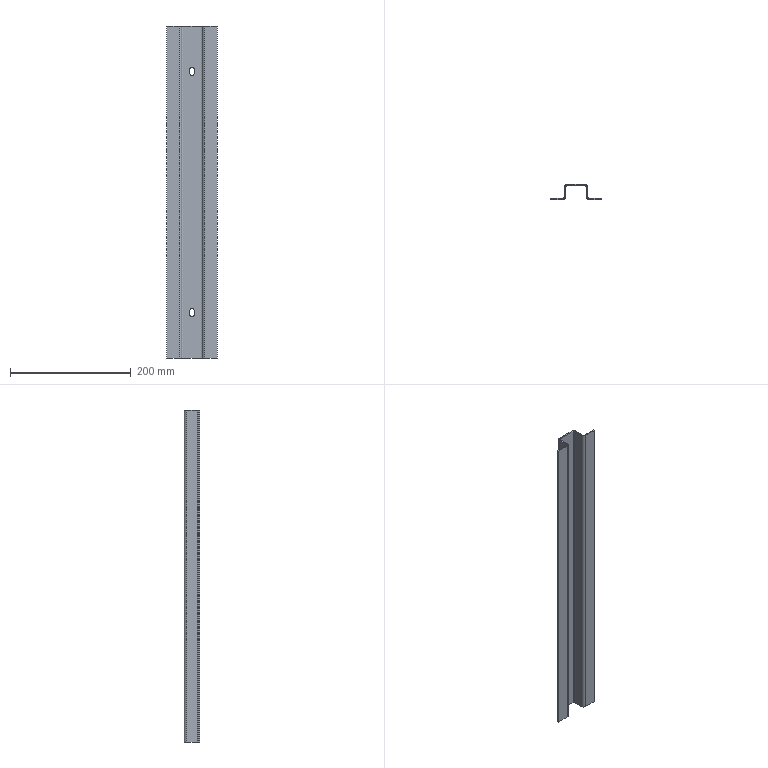Part | STEP file | SYL_0392D6J1SYL0380DJ1006_2_1-2 | 1 solid | 50 faces | box 84 x 25 x 550 mm | volume 136985 mm3 | plane 34 | cylinder 16 | commonest cylinder face diameters 7 x8 4 x4 8 x4
STEP:
#1=CARTESIAN_POINT('',(-3.5,25.,-203.5));
#2=VERTEX_POINT('',#1);
#3=CARTESIAN_POINT('',(-3.5,23.,-203.5));
#4=VERTEX_POINT('',#3);
#5=CARTESIAN_POINT('',(-3.5,23.,-203.5));
#6=DIRECTION('',(0.,-1.,0.));
#7=VECTOR('',#6,1000.);
#8=LINE('',#5,#7);
#9=EDGE_CURVE('',#2,#4,#8,.T.);
#10=ORIENTED_EDGE('',*,*,#9,.F.);
#11=CARTESIAN_POINT('',(-3.5,25.,-196.5));
#12=VERTEX_POINT('',#11);
#13=CARTESIAN_POINT('',(-3.5,25.,-275.));
#14=DIRECTION('',(0.,0.,-1.));
#15=VECTOR('',#14,1000.);
#16=LINE('',#13,#15);
#17=EDGE_CURVE('',#12,#2,#16,.T.);
#18=ORIENTED_EDGE('',*,*,#17,.F.);
#19=CARTESIAN_POINT('',(-3.5,23.,-196.5));
#20=VERTEX_POINT('',#19);
#21=CARTESIAN_POINT('',(-3.5,23.,-196.5));
#22=DIRECTION('',(0.,-1.,0.));
#23=VECTOR('',#22,1000.);
#24=LINE('',#21,#23);
#25=EDGE_CURVE('',#12,#20,#24,.T.);
#26=ORIENTED_EDGE('',*,*,#25,.T.);
#27=CARTESIAN_POINT('',(-3.5,23.,-196.5));
#28=DIRECTION('',(0.,0.,-1.));
#29=VECTOR('',#28,1000.);
#30=LINE('',#27,#29);
#31=EDGE_CURVE('',#20,#4,#30,.T.);
#32=ORIENTED_EDGE('',*,*,#31,.T.);
#33=EDGE_LOOP('',(#10,#18,#26,#32));
#34=FACE_OUTER_BOUND('',#33,.T.);
#35=CARTESIAN_POINT('',(-3.5,23.,-196.5));
#36=DIRECTION('',(-1.,0.,0.));
#37=DIRECTION('',(0.,0.,-1.));
#38=AXIS2_PLACEMENT_3D('',#35,#36,#37);
#39=PLANE('',#38);
#40=ADVANCED_FACE('',(#34),#39,.F.);
#41=ORIENTED_EDGE('',*,*,#25,.F.);
#42=CARTESIAN_POINT('',(0.,25.,-193.));
#43=VERTEX_POINT('',#42);
#44=CARTESIAN_POINT('',(0.,25.,-196.5));
#45=DIRECTION('',(0.,1.,0.));
#46=DIRECTION('',(0.,0.,1.));
#47=AXIS2_PLACEMENT_3D('',#44,#45,#46);
#48=CIRCLE('',#47,3.5);
#49=EDGE_CURVE('',#12,#43,#48,.T.);
#50=ORIENTED_EDGE('',*,*,#49,.T.);
#51=CARTESIAN_POINT('',(0.,23.,-193.));
#52=VERTEX_POINT('',#51);
#53=CARTESIAN_POINT('',(0.,23.,-193.));
#54=DIRECTION('',(0.,-1.,0.));
#55=VECTOR('',#54,1000.);
#56=LINE('',#53,#55);
#57=EDGE_CURVE('',#43,#52,#56,.T.);
#58=ORIENTED_EDGE('',*,*,#57,.T.);
#59=CARTESIAN_POINT('',(0.,23.,-196.5));
#60=DIRECTION('',(0.,1.,0.));
#61=DIRECTION('',(-1.,0.,0.));
#62=AXIS2_PLACEMENT_3D('',#59,#60,#61);
#63=CIRCLE('',#62,3.5);
#64=EDGE_CURVE('',#20,#52,#63,.T.);
#65=ORIENTED_EDGE('',*,*,#64,.F.);
#66=EDGE_LOOP('',(#41,#50,#58,#65));
#67=FACE_OUTER_BOUND('',#66,.T.);
#68=CARTESIAN_POINT('',(0.,23.,-196.5));
#69=DIRECTION('',(0.,-1.,0.));
#70=DIRECTION('',(0.,0.,-1.));
#71=AXIS2_PLACEMENT_3D('',#68,#69,#70);
#72=CYLINDRICAL_SURFACE('',#71,3.5);
#73=ADVANCED_FACE('',(#67),#72,.F.);
#74=ORIENTED_EDGE('',*,*,#57,.F.);
#75=CARTESIAN_POINT('',(3.5,25.,-196.5));
#76=VERTEX_POINT('',#75);
#77=CARTESIAN_POINT('',(0.,25.,-196.5));
#78=DIRECTION('',(0.,1.,0.));
#79=DIRECTION('',(0.,0.,1.));
#80=AXIS2_PLACEMENT_3D('',#77,#78,#79);
#81=CIRCLE('',#80,3.5);
#82=EDGE_CURVE('',#43,#76,#81,.T.);
#83=ORIENTED_EDGE('',*,*,#82,.T.);
#84=CARTESIAN_POINT('',(3.5,23.,-196.5));
#85=VERTEX_POINT('',#84);
#86=CARTESIAN_POINT('',(3.5,23.,-196.5));
#87=DIRECTION('',(0.,-1.,0.));
#88=VECTOR('',#87,1000.);
#89=LINE('',#86,#88);
#90=EDGE_CURVE('',#76,#85,#89,.T.);
#91=ORIENTED_EDGE('',*,*,#90,.T.);
#92=CARTESIAN_POINT('',(0.,23.,-196.5));
#93=DIRECTION('',(0.,1.,0.));
#94=DIRECTION('',(0.,0.,1.));
#95=AXIS2_PLACEMENT_3D('',#92,#93,#94);
#96=CIRCLE('',#95,3.5);
#97=EDGE_CURVE('',#52,#85,#96,.T.);
#98=ORIENTED_EDGE('',*,*,#97,.F.);
#99=EDGE_LOOP('',(#74,#83,#91,#98));
#100=FACE_OUTER_BOUND('',#99,.T.);
#101=CARTESIAN_POINT('',(0.,23.,-196.5));
#102=DIRECTION('',(0.,-1.,0.));
#103=DIRECTION('',(0.,0.,-1.));
#104=AXIS2_PLACEMENT_3D('',#101,#102,#103);
#105=CYLINDRICAL_SURFACE('',#104,3.5);
#106=ADVANCED_FACE('',(#100),#105,.F.);
#107=ORIENTED_EDGE('',*,*,#90,.F.);
#108=CARTESIAN_POINT('',(3.5,25.,-203.5));
#109=VERTEX_POINT('',#108);
#110=CARTESIAN_POINT('',(3.5,25.,-275.));
#111=DIRECTION('',(0.,0.,1.));
#112=VECTOR('',#111,1000.);
#113=LINE('',#110,#112);
#114=EDGE_CURVE('',#109,#76,#113,.T.);
#115=ORIENTED_EDGE('',*,*,#114,.F.);
#116=CARTESIAN_POINT('',(3.5,23.,-203.5));
#117=VERTEX_POINT('',#116);
#118=CARTESIAN_POINT('',(3.5,23.,-203.5));
#119=DIRECTION('',(0.,-1.,0.));
#120=VECTOR('',#119,1000.);
#121=LINE('',#118,#120);
#122=EDGE_CURVE('',#109,#117,#121,.T.);
#123=ORIENTED_EDGE('',*,*,#122,.T.);
#124=CARTESIAN_POINT('',(3.5,23.,-203.5));
#125=DIRECTION('',(0.,0.,1.));
#126=VECTOR('',#125,1000.);
#127=LINE('',#124,#126);
#128=EDGE_CURVE('',#117,#85,#127,.T.);
#129=ORIENTED_EDGE('',*,*,#128,.T.);
#130=EDGE_LOOP('',(#107,#115,#123,#129));
#131=FACE_OUTER_BOUND('',#130,.T.);
#132=CARTESIAN_POINT('',(3.5,23.,-203.5));
#133=DIRECTION('',(1.,0.,0.));
#134=DIRECTION('',(0.,0.,1.));
#135=AXIS2_PLACEMENT_3D('',#132,#133,#134);
#136=PLANE('',#135);
#137=ADVANCED_FACE('',(#131),#136,.F.);
#138=ORIENTED_EDGE('',*,*,#122,.F.);
#139=CARTESIAN_POINT('',(0.,25.,-207.));
#140=VERTEX_POINT('',#139);
#141=CARTESIAN_POINT('',(0.,25.,-203.5));
#142=DIRECTION('',(0.,1.,0.));
#143=DIRECTION('',(0.,0.,1.));
#144=AXIS2_PLACEMENT_3D('',#141,#142,#143);
#145=CIRCLE('',#144,3.5);
#146=EDGE_CURVE('',#109,#140,#145,.T.);
#147=ORIENTED_EDGE('',*,*,#146,.T.);
#148=CARTESIAN_POINT('',(0.,23.,-207.));
#149=VERTEX_POINT('',#148);
#150=CARTESIAN_POINT('',(0.,23.,-207.));
#151=DIRECTION('',(0.,-1.,0.));
#152=VECTOR('',#151,1000.);
#153=LINE('',#150,#152);
#154=EDGE_CURVE('',#140,#149,#153,.T.);
#155=ORIENTED_EDGE('',*,*,#154,.T.);
#156=CARTESIAN_POINT('',(0.,23.,-203.5));
#157=DIRECTION('',(0.,1.,0.));
#158=DIRECTION('',(1.,0.,0.));
#159=AXIS2_PLACEMENT_3D('',#156,#157,#158);
#160=CIRCLE('',#159,3.5);
#161=EDGE_CURVE('',#117,#149,#160,.T.);
#162=ORIENTED_EDGE('',*,*,#161,.F.);
#163=EDGE_LOOP('',(#138,#147,#155,#162));
#164=FACE_OUTER_BOUND('',#163,.T.);
#165=CARTESIAN_POINT('',(0.,23.,-203.5));
#166=DIRECTION('',(0.,-1.,0.));
#167=DIRECTION('',(0.,0.,-1.));
#168=AXIS2_PLACEMENT_3D('',#165,#166,#167);
#169=CYLINDRICAL_SURFACE('',#168,3.5);
#170=ADVANCED_FACE('',(#164),#169,.F.);
#171=CARTESIAN_POINT('',(-3.5,25.,196.5));
#172=VERTEX_POINT('',#171);
#173=CARTESIAN_POINT('',(-3.5,23.,196.5));
#174=VERTEX_POINT('',#173);
#175=CARTESIAN_POINT('',(-3.5,23.,196.5));
#176=DIRECTION('',(0.,-1.,0.));
#177=VECTOR('',#176,1000.);
#178=LINE('',#175,#177);
#179=EDGE_CURVE('',#172,#174,#178,.T.);
#180=ORIENTED_EDGE('',*,*,#179,.F.);
#181=CARTESIAN_POINT('',(-3.5,25.,203.5));
#182=VERTEX_POINT('',#181);
#183=CARTESIAN_POINT('',(-3.5,25.,-275.));
#184=DIRECTION('',(0.,0.,-1.));
#185=VECTOR('',#184,1000.);
#186=LINE('',#183,#185);
#187=EDGE_CURVE('',#182,#172,#186,.T.);
#188=ORIENTED_EDGE('',*,*,#187,.F.);
#189=CARTESIAN_POINT('',(-3.5,23.,203.5));
#190=VERTEX_POINT('',#189);
#191=CARTESIAN_POINT('',(-3.5,23.,203.5));
#192=DIRECTION('',(0.,-1.,0.));
#193=VECTOR('',#192,1000.);
#194=LINE('',#191,#193);
#195=EDGE_CURVE('',#182,#190,#194,.T.);
#196=ORIENTED_EDGE('',*,*,#195,.T.);
#197=CARTESIAN_POINT('',(-3.5,23.,203.5));
#198=DIRECTION('',(0.,0.,-1.));
#199=VECTOR('',#198,1000.);
#200=LINE('',#197,#199);
#201=EDGE_CURVE('',#190,#174,#200,.T.);
#202=ORIENTED_EDGE('',*,*,#201,.T.);
#203=EDGE_LOOP('',(#180,#188,#196,#202));
#204=FACE_OUTER_BOUND('',#203,.T.);
#205=CARTESIAN_POINT('',(-3.5,23.,203.5));
#206=DIRECTION('',(-1.,0.,0.));
#207=DIRECTION('',(0.,0.,-1.));
#208=AXIS2_PLACEMENT_3D('',#205,#206,#207);
#209=PLANE('',#208);
#210=ADVANCED_FACE('',(#204),#209,.F.);
#211=ORIENTED_EDGE('',*,*,#195,.F.);
#212=CARTESIAN_POINT('',(0.,25.,207.));
#213=VERTEX_POINT('',#212);
#214=CARTESIAN_POINT('',(0.,25.,203.5));
#215=DIRECTION('',(0.,1.,0.));
#216=DIRECTION('',(0.,0.,1.));
#217=AXIS2_PLACEMENT_3D('',#214,#215,#216);
#218=CIRCLE('',#217,3.5);
#219=EDGE_CURVE('',#182,#213,#218,.T.);
#220=ORIENTED_EDGE('',*,*,#219,.T.);
#221=CARTESIAN_POINT('',(0.,23.,207.));
#222=VERTEX_POINT('',#221);
#223=CARTESIAN_POINT('',(0.,23.,207.));
#224=DIRECTION('',(0.,-1.,0.));
#225=VECTOR('',#224,1000.);
#226=LINE('',#223,#225);
#227=EDGE_CURVE('',#213,#222,#226,.T.);
#228=ORIENTED_EDGE('',*,*,#227,.T.);
#229=CARTESIAN_POINT('',(0.,23.,203.5));
#230=DIRECTION('',(0.,1.,0.));
#231=DIRECTION('',(-1.,0.,0.));
#232=AXIS2_PLACEMENT_3D('',#229,#230,#231);
#233=CIRCLE('',#232,3.5);
#234=EDGE_CURVE('',#190,#222,#233,.T.);
#235=ORIENTED_EDGE('',*,*,#234,.F.);
#236=EDGE_LOOP('',(#211,#220,#228,#235));
#237=FACE_OUTER_BOUND('',#236,.T.);
#238=CARTESIAN_POINT('',(0.,23.,203.5));
#239=DIRECTION('',(0.,-1.,0.));
#240=DIRECTION('',(0.,0.,-1.));
#241=AXIS2_PLACEMENT_3D('',#238,#239,#240);
#242=CYLINDRICAL_SURFACE('',#241,3.5);
#243=ADVANCED_FACE('',(#237),#242,.F.);
#244=ORIENTED_EDGE('',*,*,#227,.F.);
#245=CARTESIAN_POINT('',(3.5,25.,203.5));
#246=VERTEX_POINT('',#245);
#247=CARTESIAN_POINT('',(0.,25.,203.5));
#248=DIRECTION('',(0.,1.,0.));
#249=DIRECTION('',(0.,0.,1.));
#250=AXIS2_PLACEMENT_3D('',#247,#248,#249);
#251=CIRCLE('',#250,3.5);
#252=EDGE_CURVE('',#213,#246,#251,.T.);
#253=ORIENTED_EDGE('',*,*,#252,.T.);
#254=CARTESIAN_POINT('',(3.5,23.,203.5));
#255=VERTEX_POINT('',#254);
#256=CARTESIAN_POINT('',(3.5,23.,203.5));
#257=DIRECTION('',(0.,-1.,0.));
#258=VECTOR('',#257,1000.);
#259=LINE('',#256,#258);
#260=EDGE_CURVE('',#246,#255,#259,.T.);
#261=ORIENTED_EDGE('',*,*,#260,.T.);
#262=CARTESIAN_POINT('',(0.,23.,203.5));
#263=DIRECTION('',(0.,1.,0.));
#264=DIRECTION('',(0.,0.,1.));
#265=AXIS2_PLACEMENT_3D('',#262,#263,#264);
#266=CIRCLE('',#265,3.5);
#267=EDGE_CURVE('',#222,#255,#266,.T.);
#268=ORIENTED_EDGE('',*,*,#267,.F.);
#269=EDGE_LOOP('',(#244,#253,#261,#268));
#270=FACE_OUTER_BOUND('',#269,.T.);
#271=CARTESIAN_POINT('',(0.,23.,203.5));
#272=DIRECTION('',(0.,-1.,0.));
#273=DIRECTION('',(0.,0.,-1.));
#274=AXIS2_PLACEMENT_3D('',#271,#272,#273);
#275=CYLINDRICAL_SURFACE('',#274,3.5);
#276=ADVANCED_FACE('',(#270),#275,.F.);
#277=ORIENTED_EDGE('',*,*,#260,.F.);
#278=CARTESIAN_POINT('',(3.5,25.,196.5));
#279=VERTEX_POINT('',#278);
#280=CARTESIAN_POINT('',(3.5,25.,-275.));
#281=DIRECTION('',(0.,0.,1.));
#282=VECTOR('',#281,1000.);
#283=LINE('',#280,#282);
#284=EDGE_CURVE('',#279,#246,#283,.T.);
#285=ORIENTED_EDGE('',*,*,#284,.F.);
#286=CARTESIAN_POINT('',(3.5,23.,196.5));
#287=VERTEX_POINT('',#286);
#288=CARTESIAN_POINT('',(3.5,23.,196.5));
#289=DIRECTION('',(0.,-1.,0.));
#290=VECTOR('',#289,1000.);
#291=LINE('',#288,#290);
#292=EDGE_CURVE('',#279,#287,#291,.T.);
#293=ORIENTED_EDGE('',*,*,#292,.T.);
#294=CARTESIAN_POINT('',(3.5,23.,196.5));
#295=DIRECTION('',(0.,0.,1.));
#296=VECTOR('',#295,1000.);
#297=LINE('',#294,#296);
#298=EDGE_CURVE('',#287,#255,#297,.T.);
#299=ORIENTED_EDGE('',*,*,#298,.T.);
#300=EDGE_LOOP('',(#277,#285,#293,#299));
#301=FACE_OUTER_BOUND('',#300,.T.);
#302=CARTESIAN_POINT('',(3.5,23.,196.5));
#303=DIRECTION('',(1.,0.,0.));
#304=DIRECTION('',(0.,0.,1.));
#305=AXIS2_PLACEMENT_3D('',#302,#303,#304);
#306=PLANE('',#305);
#307=ADVANCED_FACE('',(#301),#306,.F.);
#308=ORIENTED_EDGE('',*,*,#292,.F.);
#309=CARTESIAN_POINT('',(0.,25.,193.));
#310=VERTEX_POINT('',#309);
#311=CARTESIAN_POINT('',(0.,25.,196.5));
#312=DIRECTION('',(0.,1.,0.));
#313=DIRECTION('',(0.,0.,1.));
#314=AXIS2_PLACEMENT_3D('',#311,#312,#313);
#315=CIRCLE('',#314,3.5);
#316=EDGE_CURVE('',#279,#310,#315,.T.);
#317=ORIENTED_EDGE('',*,*,#316,.T.);
#318=CARTESIAN_POINT('',(0.,23.,193.));
#319=VERTEX_POINT('',#318);
#320=CARTESIAN_POINT('',(0.,23.,193.));
#321=DIRECTION('',(0.,-1.,0.));
#322=VECTOR('',#321,1000.);
#323=LINE('',#320,#322);
#324=EDGE_CURVE('',#310,#319,#323,.T.);
#325=ORIENTED_EDGE('',*,*,#324,.T.);
#326=CARTESIAN_POINT('',(0.,23.,196.5));
#327=DIRECTION('',(0.,1.,0.));
#328=DIRECTION('',(1.,0.,0.));
#329=AXIS2_PLACEMENT_3D('',#326,#327,#328);
#330=CIRCLE('',#329,3.5);
#331=EDGE_CURVE('',#287,#319,#330,.T.);
#332=ORIENTED_EDGE('',*,*,#331,.F.);
#333=EDGE_LOOP('',(#308,#317,#325,#332));
#334=FACE_OUTER_BOUND('',#333,.T.);
#335=CARTESIAN_POINT('',(0.,23.,196.5));
#336=DIRECTION('',(0.,-1.,0.));
#337=DIRECTION('',(0.,0.,-1.));
#338=AXIS2_PLACEMENT_3D('',#335,#336,#337);
#339=CYLINDRICAL_SURFACE('',#338,3.5);
#340=ADVANCED_FACE('',(#334),#339,.F.);
#341=CARTESIAN_POINT('',(-19.,21.,-275.));
#342=VERTEX_POINT('',#341);
#343=CARTESIAN_POINT('',(-17.,21.,-275.));
#344=VERTEX_POINT('',#343);
#345=CARTESIAN_POINT('',(-17.,21.,-275.));
#346=DIRECTION('',(1.,0.,0.));
#347=VECTOR('',#346,1000.);
#348=LINE('',#345,#347);
#349=EDGE_CURVE('',#342,#344,#348,.T.);
#350=ORIENTED_EDGE('',*,*,#349,.F.);
#351=CARTESIAN_POINT('',(-15.,25.,-275.));
#352=VERTEX_POINT('',#351);
#353=CARTESIAN_POINT('',(-15.,21.,-275.));
#354=DIRECTION('',(0.,0.,1.));
#355=DIRECTION('',(1.,0.,0.));
#356=AXIS2_PLACEMENT_3D('',#353,#354,#355);
#357=CIRCLE('',#356,4.);
#358=EDGE_CURVE('',#352,#342,#357,.T.);
#359=ORIENTED_EDGE('',*,*,#358,.F.);
#360=CARTESIAN_POINT('',(-15.,23.,-275.));
#361=VERTEX_POINT('',#360);
#362=CARTESIAN_POINT('',(-15.,23.,-275.));
#363=DIRECTION('',(0.,-1.,0.));
#364=VECTOR('',#363,1000.);
#365=LINE('',#362,#364);
#366=EDGE_CURVE('',#352,#361,#365,.T.);
#367=ORIENTED_EDGE('',*,*,#366,.T.);
#368=CARTESIAN_POINT('',(-15.,21.,-275.));
#369=DIRECTION('',(0.,0.,1.));
#370=DIRECTION('',(0.,1.,0.));
#371=AXIS2_PLACEMENT_3D('',#368,#369,#370);
#372=CIRCLE('',#371,2.);
#373=EDGE_CURVE('',#361,#344,#372,.T.);
#374=ORIENTED_EDGE('',*,*,#373,.T.);
#375=EDGE_LOOP('',(#350,#359,#367,#374));
#376=FACE_OUTER_BOUND('',#375,.T.);
#377=CARTESIAN_POINT('',(-15.,21.,-275.));
#378=DIRECTION('',(0.,0.,-1.));
#379=DIRECTION('',(-1.,0.,0.));
#380=AXIS2_PLACEMENT_3D('',#377,#378,#379);
#381=PLANE('',#380);
#382=ADVANCED_FACE('',(#376),#381,.T.);
#383=ORIENTED_EDGE('',*,*,#366,.F.);
#384=CARTESIAN_POINT('',(15.,25.,-275.));
#385=VERTEX_POINT('',#384);
#386=CARTESIAN_POINT('',(-15.,25.,-275.));
#387=DIRECTION('',(-1.,0.,0.));
#388=VECTOR('',#387,1000.);
#389=LINE('',#386,#388);
#390=EDGE_CURVE('',#385,#352,#389,.T.);
#391=ORIENTED_EDGE('',*,*,#390,.F.);
#392=CARTESIAN_POINT('',(15.,23.,-275.));
#393=VERTEX_POINT('',#392);
#394=CARTESIAN_POINT('',(15.,23.,-275.));
#395=DIRECTION('',(0.,-1.,0.));
#396=VECTOR('',#395,1000.);
#397=LINE('',#394,#396);
#398=EDGE_CURVE('',#385,#393,#397,.T.);
#399=ORIENTED_EDGE('',*,*,#398,.T.);
#400=CARTESIAN_POINT('',(15.,23.,-275.));
#401=DIRECTION('',(-1.,0.,0.));
#402=VECTOR('',#401,1000.);
#403=LINE('',#400,#402);
#404=EDGE_CURVE('',#393,#361,#403,.T.);
#405=ORIENTED_EDGE('',*,*,#404,.T.);
#406=EDGE_LOOP('',(#383,#391,#399,#405));
#407=FACE_OUTER_BOUND('',#406,.T.);
#408=CARTESIAN_POINT('',(15.,23.,-275.));
#409=DIRECTION('',(0.,0.,1.));
#410=DIRECTION('',(-1.,0.,0.));
#411=AXIS2_PLACEMENT_3D('',#408,#409,#410);
#412=PLANE('',#411);
#413=ADVANCED_FACE('',(#407),#412,.F.);
#414=ORIENTED_EDGE('',*,*,#398,.F.);
#415=CARTESIAN_POINT('',(19.,21.,-275.));
#416=VERTEX_POINT('',#415);
#417=CARTESIAN_POINT('',(15.,21.,-275.));
#418=DIRECTION('',(0.,0.,1.));
#419=DIRECTION('',(1.,0.,0.));
#420=AXIS2_PLACEMENT_3D('',#417,#418,#419);
#421=CIRCLE('',#420,4.);
#422=EDGE_CURVE('',#416,#385,#421,.T.);
#423=ORIENTED_EDGE('',*,*,#422,.F.);
#424=CARTESIAN_POINT('',(17.,21.,-275.));
#425=VERTEX_POINT('',#424);
#426=CARTESIAN_POINT('',(17.,21.,-275.));
#427=DIRECTION('',(-1.,0.,0.));
#428=VECTOR('',#427,1000.);
#429=LINE('',#426,#428);
#430=EDGE_CURVE('',#416,#425,#429,.T.);
#431=ORIENTED_EDGE('',*,*,#430,.T.);
#432=CARTESIAN_POINT('',(15.,21.,-275.));
#433=DIRECTION('',(0.,0.,1.));
#434=DIRECTION('',(1.,0.,0.));
#435=AXIS2_PLACEMENT_3D('',#432,#433,#434);
#436=CIRCLE('',#435,2.);
#437=EDGE_CURVE('',#425,#393,#436,.T.);
#438=ORIENTED_EDGE('',*,*,#437,.T.);
#439=EDGE_LOOP('',(#414,#423,#431,#438));
#440=FACE_OUTER_BOUND('',#439,.T.);
#441=CARTESIAN_POINT('',(15.,21.,-275.));
#442=DIRECTION('',(0.,0.,-1.));
#443=DIRECTION('',(-1.,0.,0.));
#444=AXIS2_PLACEMENT_3D('',#441,#442,#443);
#445=PLANE('',#444);
#446=ADVANCED_FACE('',(#440),#445,.T.);
#447=ORIENTED_EDGE('',*,*,#430,.F.);
#448=CARTESIAN_POINT('',(19.,4.,-275.));
#449=VERTEX_POINT('',#448);
#450=CARTESIAN_POINT('',(19.,21.,-275.));
#451=DIRECTION('',(0.,1.,0.));
#452=VECTOR('',#451,1000.);
#453=LINE('',#450,#452);
#454=EDGE_CURVE('',#449,#416,#453,.T.);
#455=ORIENTED_EDGE('',*,*,#454,.F.);
#456=CARTESIAN_POINT('',(17.,4.,-275.));
#457=VERTEX_POINT('',#456);
#458=CARTESIAN_POINT('',(17.,4.,-275.));
#459=DIRECTION('',(-1.,0.,0.));
#460=VECTOR('',#459,1000.);
#461=LINE('',#458,#460);
#462=EDGE_CURVE('',#449,#457,#461,.T.);
#463=ORIENTED_EDGE('',*,*,#462,.T.);
#464=CARTESIAN_POINT('',(17.,4.,-275.));
#465=DIRECTION('',(0.,1.,0.));
#466=VECTOR('',#465,1000.);
#467=LINE('',#464,#466);
#468=EDGE_CURVE('',#457,#425,#467,.T.);
#469=ORIENTED_EDGE('',*,*,#468,.T.);
#470=EDGE_LOOP('',(#447,#455,#463,#469));
#471=FACE_OUTER_BOUND('',#470,.T.);
#472=CARTESIAN_POINT('',(17.,4.,-275.));
#473=DIRECTION('',(0.,0.,1.));
#474=DIRECTION('',(0.,1.,0.));
#475=AXIS2_PLACEMENT_3D('',#472,#473,#474);
#476=PLANE('',#475);
#477=ADVANCED_FACE('',(#471),#476,.F.);
#478=ORIENTED_EDGE('',*,*,#462,.F.);
#479=CARTESIAN_POINT('',(21.,2.,-275.));
#480=VERTEX_POINT('',#479);
#481=CARTESIAN_POINT('',(21.,4.,-275.));
#482=DIRECTION('',(0.,0.,-1.));
#483=DIRECTION('',(1.,0.,0.));
#484=AXIS2_PLACEMENT_3D('',#481,#482,#483);
#485=CIRCLE('',#484,2.);
#486=EDGE_CURVE('',#480,#449,#485,.T.);
#487=ORIENTED_EDGE('',*,*,#486,.F.);
#488=CARTESIAN_POINT('',(21.,0.,-275.));
#489=VERTEX_POINT('',#488);
#490=CARTESIAN_POINT('',(21.,0.,-275.));
#491=DIRECTION('',(0.,-1.,0.));
#492=VECTOR('',#491,1000.);
#493=LINE('',#490,#492);
#494=EDGE_CURVE('',#480,#489,#493,.T.);
#495=ORIENTED_EDGE('',*,*,#494,.T.);
#496=CARTESIAN_POINT('',(21.,4.,-275.));
#497=DIRECTION('',(0.,0.,-1.));
#498=DIRECTION('',(0.,-1.,0.));
#499=AXIS2_PLACEMENT_3D('',#496,#497,#498);
#500=CIRCLE('',#499,4.);
#501=EDGE_CURVE('',#489,#457,#500,.T.);
#502=ORIENTED_EDGE('',*,*,#501,.T.);
#503=EDGE_LOOP('',(#478,#487,#495,#502));
#504=FACE_OUTER_BOUND('',#503,.T.);
#505=CARTESIAN_POINT('',(21.,4.,-275.));
#506=DIRECTION('',(0.,0.,1.));
#507=DIRECTION('',(1.,0.,0.));
#508=AXIS2_PLACEMENT_3D('',#505,#506,#507);
#509=PLANE('',#508);
#510=ADVANCED_FACE('',(#504),#509,.F.);
#511=ORIENTED_EDGE('',*,*,#494,.F.);
#512=CARTESIAN_POINT('',(42.,2.,-275.));
#513=VERTEX_POINT('',#512);
#514=CARTESIAN_POINT('',(21.,2.,-275.));
#515=DIRECTION('',(-1.,0.,0.));
#516=VECTOR('',#515,1000.);
#517=LINE('',#514,#516);
#518=EDGE_CURVE('',#513,#480,#517,.T.);
#519=ORIENTED_EDGE('',*,*,#518,.F.);
#520=CARTESIAN_POINT('',(42.,0.,-275.));
#521=VERTEX_POINT('',#520);
#522=CARTESIAN_POINT('',(42.,0.,-275.));
#523=DIRECTION('',(0.,-1.,0.));
#524=VECTOR('',#523,1000.);
#525=LINE('',#522,#524);
#526=EDGE_CURVE('',#513,#521,#525,.T.);
#527=ORIENTED_EDGE('',*,*,#526,.T.);
#528=CARTESIAN_POINT('',(42.,0.,-275.));
#529=DIRECTION('',(-1.,0.,0.));
#530=VECTOR('',#529,1000.);
#531=LINE('',#528,#530);
#532=EDGE_CURVE('',#521,#489,#531,.T.);
#533=ORIENTED_EDGE('',*,*,#532,.T.);
#534=EDGE_LOOP('',(#511,#519,#527,#533));
#535=FACE_OUTER_BOUND('',#534,.T.);
#536=CARTESIAN_POINT('',(42.,0.,-275.));
#537=DIRECTION('',(0.,0.,1.));
#538=DIRECTION('',(-1.,0.,0.));
#539=AXIS2_PLACEMENT_3D('',#536,#537,#538);
#540=PLANE('',#539);
#541=ADVANCED_FACE('',(#535),#540,.F.);
#542=ORIENTED_EDGE('',*,*,#526,.F.);
#543=CARTESIAN_POINT('',(42.,2.,275.));
#544=VERTEX_POINT('',#543);
#545=CARTESIAN_POINT('',(42.,2.,-275.));
#546=DIRECTION('',(0.,0.,-1.));
#547=VECTOR('',#546,1000.);
#548=LINE('',#545,#547);
#549=EDGE_CURVE('',#544,#513,#548,.T.);
#550=ORIENTED_EDGE('',*,*,#549,.F.);
#551=CARTESIAN_POINT('',(42.,0.,275.));
#552=VERTEX_POINT('',#551);
#553=CARTESIAN_POINT('',(42.,0.,275.));
#554=DIRECTION('',(0.,-1.,0.));
#555=VECTOR('',#554,1000.);
#556=LINE('',#553,#555);
#557=EDGE_CURVE('',#544,#552,#556,.T.);
#558=ORIENTED_EDGE('',*,*,#557,.T.);
#559=CARTESIAN_POINT('',(42.,0.,275.));
#560=DIRECTION('',(0.,0.,-1.));
#561=VECTOR('',#560,1000.);
#562=LINE('',#559,#561);
#563=EDGE_CURVE('',#552,#521,#562,.T.);
#564=ORIENTED_EDGE('',*,*,#563,.T.);
#565=EDGE_LOOP('',(#542,#550,#558,#564));
#566=FACE_OUTER_BOUND('',#565,.T.);
#567=CARTESIAN_POINT('',(42.,0.,275.));
#568=DIRECTION('',(-1.,0.,0.));
#569=DIRECTION('',(0.,0.,-1.));
#570=AXIS2_PLACEMENT_3D('',#567,#568,#569);
#571=PLANE('',#570);
#572=ADVANCED_FACE('',(#566),#571,.F.);
#573=ORIENTED_EDGE('',*,*,#557,.F.);
#574=CARTESIAN_POINT('',(21.,2.,275.));
#575=VERTEX_POINT('',#574);
#576=CARTESIAN_POINT('',(21.,2.,275.));
#577=DIRECTION('',(1.,0.,0.));
#578=VECTOR('',#577,1000.);
#579=LINE('',#576,#578);
#580=EDGE_CURVE('',#575,#544,#579,.T.);
#581=ORIENTED_EDGE('',*,*,#580,.F.);
#582=CARTESIAN_POINT('',(21.,0.,275.));
#583=VERTEX_POINT('',#582);
#584=CARTESIAN_POINT('',(21.,0.,275.));
#585=DIRECTION('',(0.,-1.,0.));
#586=VECTOR('',#585,1000.);
#587=LINE('',#584,#586);
#588=EDGE_CURVE('',#575,#583,#587,.T.);
#589=ORIENTED_EDGE('',*,*,#588,.T.);
#590=CARTESIAN_POINT('',(21.,0.,275.));
#591=DIRECTION('',(1.,0.,0.));
#592=VECTOR('',#591,1000.);
#593=LINE('',#590,#592);
#594=EDGE_CURVE('',#583,#552,#593,.T.);
#595=ORIENTED_EDGE('',*,*,#594,.T.);
#596=EDGE_LOOP('',(#573,#581,#589,#595));
#597=FACE_OUTER_BOUND('',#596,.T.);
#598=CARTESIAN_POINT('',(21.,0.,275.));
#599=DIRECTION('',(0.,0.,-1.));
#600=DIRECTION('',(1.,0.,0.));
#601=AXIS2_PLACEMENT_3D('',#598,#599,#600);
#602=PLANE('',#601);
#603=ADVANCED_FACE('',(#597),#602,.F.);
#604=ORIENTED_EDGE('',*,*,#588,.F.);
#605=CARTESIAN_POINT('',(19.,4.,275.));
#606=VERTEX_POINT('',#605);
#607=CARTESIAN_POINT('',(21.,4.,275.));
#608=DIRECTION('',(0.,0.,1.));
#609=DIRECTION('',(1.,0.,0.));
#610=AXIS2_PLACEMENT_3D('',#607,#608,#609);
#611=CIRCLE('',#610,2.);
#612=EDGE_CURVE('',#606,#575,#611,.T.);
#613=ORIENTED_EDGE('',*,*,#612,.F.);
#614=CARTESIAN_POINT('',(17.,4.,275.));
#615=VERTEX_POINT('',#614);
#616=CARTESIAN_POINT('',(17.,4.,275.));
#617=DIRECTION('',(-1.,0.,0.));
#618=VECTOR('',#617,1000.);
#619=LINE('',#616,#618);
#620=EDGE_CURVE('',#606,#615,#619,.T.);
#621=ORIENTED_EDGE('',*,*,#620,.T.);
#622=CARTESIAN_POINT('',(21.,4.,275.));
#623=DIRECTION('',(0.,0.,1.));
#624=DIRECTION('',(-1.,0.,0.));
#625=AXIS2_PLACEMENT_3D('',#622,#623,#624);
#626=CIRCLE('',#625,4.);
#627=EDGE_CURVE('',#615,#583,#626,.T.);
#628=ORIENTED_EDGE('',*,*,#627,.T.);
#629=EDGE_LOOP('',(#604,#613,#621,#628));
#630=FACE_OUTER_BOUND('',#629,.T.);
#631=CARTESIAN_POINT('',(21.,4.,275.));
#632=DIRECTION('',(0.,0.,-1.));
#633=DIRECTION('',(-1.,0.,0.));
#634=AXIS2_PLACEMENT_3D('',#631,#632,#633);
#635=PLANE('',#634);
#636=ADVANCED_FACE('',(#630),#635,.F.);
#637=ORIENTED_EDGE('',*,*,#620,.F.);
#638=CARTESIAN_POINT('',(19.,21.,275.));
#639=VERTEX_POINT('',#638);
#640=CARTESIAN_POINT('',(19.,21.,275.));
#641=DIRECTION('',(0.,-1.,0.));
#642=VECTOR('',#641,1000.);
#643=LINE('',#640,#642);
#644=EDGE_CURVE('',#639,#606,#643,.T.);
#645=ORIENTED_EDGE('',*,*,#644,.F.);
#646=CARTESIAN_POINT('',(17.,21.,275.));
#647=VERTEX_POINT('',#646);
#648=CARTESIAN_POINT('',(17.,21.,275.));
#649=DIRECTION('',(-1.,0.,0.));
#650=VECTOR('',#649,1000.);
#651=LINE('',#648,#650);
#652=EDGE_CURVE('',#639,#647,#651,.T.);
#653=ORIENTED_EDGE('',*,*,#652,.T.);
#654=CARTESIAN_POINT('',(17.,21.,275.));
#655=DIRECTION('',(0.,-1.,0.));
#656=VECTOR('',#655,1000.);
#657=LINE('',#654,#656);
#658=EDGE_CURVE('',#647,#615,#657,.T.);
#659=ORIENTED_EDGE('',*,*,#658,.T.);
#660=EDGE_LOOP('',(#637,#645,#653,#659));
#661=FACE_OUTER_BOUND('',#660,.T.);
#662=CARTESIAN_POINT('',(17.,21.,275.));
#663=DIRECTION('',(0.,0.,-1.));
#664=DIRECTION('',(0.,-1.,0.));
#665=AXIS2_PLACEMENT_3D('',#662,#663,#664);
#666=PLANE('',#665);
#667=ADVANCED_FACE('',(#661),#666,.F.);
#668=ORIENTED_EDGE('',*,*,#652,.F.);
#669=CARTESIAN_POINT('',(15.,25.,275.));
#670=VERTEX_POINT('',#669);
#671=CARTESIAN_POINT('',(15.,21.,275.));
#672=DIRECTION('',(0.,0.,-1.));
#673=DIRECTION('',(1.,0.,0.));
#674=AXIS2_PLACEMENT_3D('',#671,#672,#673);
#675=CIRCLE('',#674,4.);
#676=EDGE_CURVE('',#670,#639,#675,.T.);
#677=ORIENTED_EDGE('',*,*,#676,.F.);
#678=CARTESIAN_POINT('',(15.,23.,275.));
#679=VERTEX_POINT('',#678);
#680=CARTESIAN_POINT('',(15.,23.,275.));
#681=DIRECTION('',(0.,-1.,0.));
#682=VECTOR('',#681,1000.);
#683=LINE('',#680,#682);
#684=EDGE_CURVE('',#670,#679,#683,.T.);
#685=ORIENTED_EDGE('',*,*,#684,.T.);
#686=CARTESIAN_POINT('',(15.,21.,275.));
#687=DIRECTION('',(0.,0.,-1.));
#688=DIRECTION('',(0.,1.,0.));
#689=AXIS2_PLACEMENT_3D('',#686,#687,#688);
#690=CIRCLE('',#689,2.);
#691=EDGE_CURVE('',#679,#647,#690,.T.);
#692=ORIENTED_EDGE('',*,*,#691,.T.);
#693=EDGE_LOOP('',(#668,#677,#685,#692));
#694=FACE_OUTER_BOUND('',#693,.T.);
#695=CARTESIAN_POINT('',(15.,21.,275.));
#696=DIRECTION('',(0.,0.,1.));
#697=DIRECTION('',(1.,0.,0.));
#698=AXIS2_PLACEMENT_3D('',#695,#696,#697);
#699=PLANE('',#698);
#700=ADVANCED_FACE('',(#694),#699,.T.);
#701=ORIENTED_EDGE('',*,*,#684,.F.);
#702=CARTESIAN_POINT('',(-15.,25.,275.));
#703=VERTEX_POINT('',#702);
#704=CARTESIAN_POINT('',(-15.,25.,275.));
#705=DIRECTION('',(1.,0.,0.));
#706=VECTOR('',#705,1000.);
#707=LINE('',#704,#706);
#708=EDGE_CURVE('',#703,#670,#707,.T.);
#709=ORIENTED_EDGE('',*,*,#708,.F.);
#710=CARTESIAN_POINT('',(-15.,23.,275.));
#711=VERTEX_POINT('',#710);
#712=CARTESIAN_POINT('',(-15.,23.,275.));
#713=DIRECTION('',(0.,-1.,0.));
#714=VECTOR('',#713,1000.);
#715=LINE('',#712,#714);
#716=EDGE_CURVE('',#703,#711,#715,.T.);
#717=ORIENTED_EDGE('',*,*,#716,.T.);
#718=CARTESIAN_POINT('',(-15.,23.,275.));
#719=DIRECTION('',(1.,0.,0.));
#720=VECTOR('',#719,1000.);
#721=LINE('',#718,#720);
#722=EDGE_CURVE('',#711,#679,#721,.T.);
#723=ORIENTED_EDGE('',*,*,#722,.T.);
#724=EDGE_LOOP('',(#701,#709,#717,#723));
#725=FACE_OUTER_BOUND('',#724,.T.);
#726=CARTESIAN_POINT('',(-15.,23.,275.));
#727=DIRECTION('',(0.,0.,-1.));
#728=DIRECTION('',(1.,0.,0.));
#729=AXIS2_PLACEMENT_3D('',#726,#727,#728);
#730=PLANE('',#729);
#731=ADVANCED_FACE('',(#725),#730,.F.);
#732=ORIENTED_EDGE('',*,*,#716,.F.);
#733=CARTESIAN_POINT('',(-19.,21.,275.));
#734=VERTEX_POINT('',#733);
#735=CARTESIAN_POINT('',(-15.,21.,275.));
#736=DIRECTION('',(0.,0.,-1.));
#737=DIRECTION('',(1.,0.,0.));
#738=AXIS2_PLACEMENT_3D('',#735,#736,#737);
#739=CIRCLE('',#738,4.);
#740=EDGE_CURVE('',#734,#703,#739,.T.);
#741=ORIENTED_EDGE('',*,*,#740,.F.);
#742=CARTESIAN_POINT('',(-17.,21.,275.));
#743=VERTEX_POINT('',#742);
#744=CARTESIAN_POINT('',(-17.,21.,275.));
#745=DIRECTION('',(1.,0.,0.));
#746=VECTOR('',#745,1000.);
#747=LINE('',#744,#746);
#748=EDGE_CURVE('',#734,#743,#747,.T.);
#749=ORIENTED_EDGE('',*,*,#748,.T.);
#750=CARTESIAN_POINT('',(-15.,21.,275.));
#751=DIRECTION('',(0.,0.,-1.));
#752=DIRECTION('',(-1.,0.,0.));
#753=AXIS2_PLACEMENT_3D('',#750,#751,#752);
#754=CIRCLE('',#753,2.);
#755=EDGE_CURVE('',#743,#711,#754,.T.);
#756=ORIENTED_EDGE('',*,*,#755,.T.);
#757=EDGE_LOOP('',(#732,#741,#749,#756));
#758=FACE_OUTER_BOUND('',#757,.T.);
#759=CARTESIAN_POINT('',(-15.,21.,275.));
#760=DIRECTION('',(0.,0.,1.));
#761=DIRECTION('',(1.,0.,0.));
#762=AXIS2_PLACEMENT_3D('',#759,#760,#761);
#763=PLANE('',#762);
#764=ADVANCED_FACE('',(#758),#763,.T.);
#765=ORIENTED_EDGE('',*,*,#748,.F.);
#766=CARTESIAN_POINT('',(-19.,4.,275.));
#767=VERTEX_POINT('',#766);
#768=CARTESIAN_POINT('',(-19.,4.,275.));
#769=DIRECTION('',(0.,1.,0.));
#770=VECTOR('',#769,1000.);
#771=LINE('',#768,#770);
#772=EDGE_CURVE('',#767,#734,#771,.T.);
#773=ORIENTED_EDGE('',*,*,#772,.F.);
#774=CARTESIAN_POINT('',(-17.,4.,275.));
#775=VERTEX_POINT('',#774);
#776=CARTESIAN_POINT('',(-17.,4.,275.));
#777=DIRECTION('',(1.,0.,0.));
#778=VECTOR('',#777,1000.);
#779=LINE('',#776,#778);
#780=EDGE_CURVE('',#767,#775,#779,.T.);
#781=ORIENTED_EDGE('',*,*,#780,.T.);
#782=CARTESIAN_POINT('',(-17.,4.,275.));
#783=DIRECTION('',(0.,1.,0.));
#784=VECTOR('',#783,1000.);
#785=LINE('',#782,#784);
#786=EDGE_CURVE('',#775,#743,#785,.T.);
#787=ORIENTED_EDGE('',*,*,#786,.T.);
#788=EDGE_LOOP('',(#765,#773,#781,#787));
#789=FACE_OUTER_BOUND('',#788,.T.);
#790=CARTESIAN_POINT('',(-17.,4.,275.));
#791=DIRECTION('',(0.,0.,-1.));
#792=DIRECTION('',(0.,1.,0.));
#793=AXIS2_PLACEMENT_3D('',#790,#791,#792);
#794=PLANE('',#793);
#795=ADVANCED_FACE('',(#789),#794,.F.);
#796=ORIENTED_EDGE('',*,*,#780,.F.);
#797=CARTESIAN_POINT('',(-21.,2.,275.));
#798=VERTEX_POINT('',#797);
#799=CARTESIAN_POINT('',(-21.,4.,275.));
#800=DIRECTION('',(0.,0.,1.));
#801=DIRECTION('',(1.,0.,0.));
#802=AXIS2_PLACEMENT_3D('',#799,#800,#801);
#803=CIRCLE('',#802,2.);
#804=EDGE_CURVE('',#798,#767,#803,.T.);
#805=ORIENTED_EDGE('',*,*,#804,.F.);
#806=CARTESIAN_POINT('',(-21.,0.,275.));
#807=VERTEX_POINT('',#806);
#808=CARTESIAN_POINT('',(-21.,0.,275.));
#809=DIRECTION('',(0.,-1.,0.));
#810=VECTOR('',#809,1000.);
#811=LINE('',#808,#810);
#812=EDGE_CURVE('',#798,#807,#811,.T.);
#813=ORIENTED_EDGE('',*,*,#812,.T.);
#814=CARTESIAN_POINT('',(-21.,4.,275.));
#815=DIRECTION('',(0.,0.,1.));
#816=DIRECTION('',(0.,-1.,0.));
#817=AXIS2_PLACEMENT_3D('',#814,#815,#816);
#818=CIRCLE('',#817,4.);
#819=EDGE_CURVE('',#807,#775,#818,.T.);
#820=ORIENTED_EDGE('',*,*,#819,.T.);
#821=EDGE_LOOP('',(#796,#805,#813,#820));
#822=FACE_OUTER_BOUND('',#821,.T.);
#823=CARTESIAN_POINT('',(-21.,4.,275.));
#824=DIRECTION('',(0.,0.,-1.));
#825=DIRECTION('',(-1.,0.,0.));
#826=AXIS2_PLACEMENT_3D('',#823,#824,#825);
#827=PLANE('',#826);
#828=ADVANCED_FACE('',(#822),#827,.F.);
#829=ORIENTED_EDGE('',*,*,#812,.F.);
#830=CARTESIAN_POINT('',(-42.,2.,275.));
#831=VERTEX_POINT('',#830);
#832=CARTESIAN_POINT('',(-42.,2.,275.));
#833=DIRECTION('',(1.,0.,0.));
#834=VECTOR('',#833,1000.);
#835=LINE('',#832,#834);
#836=EDGE_CURVE('',#831,#798,#835,.T.);
#837=ORIENTED_EDGE('',*,*,#836,.F.);
#838=CARTESIAN_POINT('',(-42.,0.,275.));
#839=VERTEX_POINT('',#838);
#840=CARTESIAN_POINT('',(-42.,0.,275.));
#841=DIRECTION('',(0.,-1.,0.));
#842=VECTOR('',#841,1000.);
#843=LINE('',#840,#842);
#844=EDGE_CURVE('',#831,#839,#843,.T.);
#845=ORIENTED_EDGE('',*,*,#844,.T.);
#846=CARTESIAN_POINT('',(-42.,0.,275.));
#847=DIRECTION('',(1.,0.,0.));
#848=VECTOR('',#847,1000.);
#849=LINE('',#846,#848);
#850=EDGE_CURVE('',#839,#807,#849,.T.);
#851=ORIENTED_EDGE('',*,*,#850,.T.);
#852=EDGE_LOOP('',(#829,#837,#845,#851));
#853=FACE_OUTER_BOUND('',#852,.T.);
#854=CARTESIAN_POINT('',(-42.,0.,275.));
#855=DIRECTION('',(0.,0.,-1.));
#856=DIRECTION('',(1.,0.,0.));
#857=AXIS2_PLACEMENT_3D('',#854,#855,#856);
#858=PLANE('',#857);
#859=ADVANCED_FACE('',(#853),#858,.F.);
#860=ORIENTED_EDGE('',*,*,#844,.F.);
#861=CARTESIAN_POINT('',(-42.,2.,-275.));
#862=VERTEX_POINT('',#861);
#863=CARTESIAN_POINT('',(-42.,2.,-275.));
#864=DIRECTION('',(0.,0.,1.));
#865=VECTOR('',#864,1000.);
#866=LINE('',#863,#865);
#867=EDGE_CURVE('',#862,#831,#866,.T.);
#868=ORIENTED_EDGE('',*,*,#867,.F.);
#869=CARTESIAN_POINT('',(-42.,0.,-275.));
#870=VERTEX_POINT('',#869);
#871=CARTESIAN_POINT('',(-42.,0.,-275.));
#872=DIRECTION('',(0.,-1.,0.));
#873=VECTOR('',#872,1000.);
#874=LINE('',#871,#873);
#875=EDGE_CURVE('',#862,#870,#874,.T.);
#876=ORIENTED_EDGE('',*,*,#875,.T.);
#877=CARTESIAN_POINT('',(-42.,0.,-275.));
#878=DIRECTION('',(0.,0.,1.));
#879=VECTOR('',#878,1000.);
#880=LINE('',#877,#879);
#881=EDGE_CURVE('',#870,#839,#880,.T.);
#882=ORIENTED_EDGE('',*,*,#881,.T.);
#883=EDGE_LOOP('',(#860,#868,#876,#882));
#884=FACE_OUTER_BOUND('',#883,.T.);
#885=CARTESIAN_POINT('',(-42.,0.,-275.));
#886=DIRECTION('',(1.,0.,0.));
#887=DIRECTION('',(0.,0.,1.));
#888=AXIS2_PLACEMENT_3D('',#885,#886,#887);
#889=PLANE('',#888);
#890=ADVANCED_FACE('',(#884),#889,.F.);
#891=ORIENTED_EDGE('',*,*,#875,.F.);
#892=CARTESIAN_POINT('',(-21.,2.,-275.));
#893=VERTEX_POINT('',#892);
#894=CARTESIAN_POINT('',(-42.,2.,-275.));
#895=DIRECTION('',(-1.,0.,0.));
#896=VECTOR('',#895,1000.);
#897=LINE('',#894,#896);
#898=EDGE_CURVE('',#893,#862,#897,.T.);
#899=ORIENTED_EDGE('',*,*,#898,.F.);
#900=CARTESIAN_POINT('',(-21.,0.,-275.));
#901=VERTEX_POINT('',#900);
#902=CARTESIAN_POINT('',(-21.,0.,-275.));
#903=DIRECTION('',(0.,-1.,0.));
#904=VECTOR('',#903,1000.);
#905=LINE('',#902,#904);
#906=EDGE_CURVE('',#893,#901,#905,.T.);
#907=ORIENTED_EDGE('',*,*,#906,.T.);
#908=CARTESIAN_POINT('',(-21.,0.,-275.));
#909=DIRECTION('',(-1.,0.,0.));
#910=VECTOR('',#909,1000.);
#911=LINE('',#908,#910);
#912=EDGE_CURVE('',#901,#870,#911,.T.);
#913=ORIENTED_EDGE('',*,*,#912,.T.);
#914=EDGE_LOOP('',(#891,#899,#907,#913));
#915=FACE_OUTER_BOUND('',#914,.T.);
#916=CARTESIAN_POINT('',(-21.,0.,-275.));
#917=DIRECTION('',(0.,0.,1.));
#918=DIRECTION('',(-1.,0.,0.));
#919=AXIS2_PLACEMENT_3D('',#916,#917,#918);
#920=PLANE('',#919);
#921=ADVANCED_FACE('',(#915),#920,.F.);
#922=ORIENTED_EDGE('',*,*,#906,.F.);
#923=CARTESIAN_POINT('',(-19.,4.,-275.));
#924=VERTEX_POINT('',#923);
#925=CARTESIAN_POINT('',(-21.,4.,-275.));
#926=DIRECTION('',(0.,0.,-1.));
#927=DIRECTION('',(1.,0.,0.));
#928=AXIS2_PLACEMENT_3D('',#925,#926,#927);
#929=CIRCLE('',#928,2.);
#930=EDGE_CURVE('',#924,#893,#929,.T.);
#931=ORIENTED_EDGE('',*,*,#930,.F.);
#932=CARTESIAN_POINT('',(-17.,4.,-275.));
#933=VERTEX_POINT('',#932);
#934=CARTESIAN_POINT('',(-17.,4.,-275.));
#935=DIRECTION('',(1.,0.,0.));
#936=VECTOR('',#935,1000.);
#937=LINE('',#934,#936);
#938=EDGE_CURVE('',#924,#933,#937,.T.);
#939=ORIENTED_EDGE('',*,*,#938,.T.);
#940=CARTESIAN_POINT('',(-21.,4.,-275.));
#941=DIRECTION('',(0.,0.,-1.));
#942=DIRECTION('',(1.,0.,0.));
#943=AXIS2_PLACEMENT_3D('',#940,#941,#942);
#944=CIRCLE('',#943,4.);
#945=EDGE_CURVE('',#933,#901,#944,.T.);
#946=ORIENTED_EDGE('',*,*,#945,.T.);
#947=EDGE_LOOP('',(#922,#931,#939,#946));
#948=FACE_OUTER_BOUND('',#947,.T.);
#949=CARTESIAN_POINT('',(-21.,4.,-275.));
#950=DIRECTION('',(0.,0.,1.));
#951=DIRECTION('',(1.,0.,0.));
#952=AXIS2_PLACEMENT_3D('',#949,#950,#951);
#953=PLANE('',#952);
#954=ADVANCED_FACE('',(#948),#953,.F.);
#955=CARTESIAN_POINT('',(0.,25.,196.5));
#956=DIRECTION('',(0.,1.,0.));
#957=DIRECTION('',(0.,0.,1.));
#958=AXIS2_PLACEMENT_3D('',#955,#956,#957);
#959=CIRCLE('',#958,3.5);
#960=EDGE_CURVE('',#310,#172,#959,.T.);
#961=ORIENTED_EDGE('',*,*,#960,.T.);
#962=ORIENTED_EDGE('',*,*,#179,.T.);
#963=CARTESIAN_POINT('',(0.,23.,196.5));
#964=DIRECTION('',(0.,1.,0.));
#965=DIRECTION('',(0.,0.,-1.));
#966=AXIS2_PLACEMENT_3D('',#963,#964,#965);
#967=CIRCLE('',#966,3.5);
#968=EDGE_CURVE('',#319,#174,#967,.T.);
#969=ORIENTED_EDGE('',*,*,#968,.F.);
#970=ORIENTED_EDGE('',*,*,#324,.F.);
#971=EDGE_LOOP('',(#961,#962,#969,#970));
#972=FACE_OUTER_BOUND('',#971,.T.);
#973=CARTESIAN_POINT('',(0.,23.,196.5));
#974=DIRECTION('',(0.,-1.,0.));
#975=DIRECTION('',(0.,0.,-1.));
#976=AXIS2_PLACEMENT_3D('',#973,#974,#975);
#977=CYLINDRICAL_SURFACE('',#976,3.5);
#978=ADVANCED_FACE('',(#972),#977,.F.);
#979=CARTESIAN_POINT('',(0.,25.,-203.5));
#980=DIRECTION('',(0.,1.,0.));
#981=DIRECTION('',(0.,0.,1.));
#982=AXIS2_PLACEMENT_3D('',#979,#980,#981);
#983=CIRCLE('',#982,3.5);
#984=EDGE_CURVE('',#140,#2,#983,.T.);
#985=ORIENTED_EDGE('',*,*,#984,.T.);
#986=ORIENTED_EDGE('',*,*,#9,.T.);
#987=CARTESIAN_POINT('',(0.,23.,-203.5));
#988=DIRECTION('',(0.,1.,0.));
#989=DIRECTION('',(0.,0.,-1.));
#990=AXIS2_PLACEMENT_3D('',#987,#988,#989);
#991=CIRCLE('',#990,3.5);
#992=EDGE_CURVE('',#149,#4,#991,.T.);
#993=ORIENTED_EDGE('',*,*,#992,.F.);
#994=ORIENTED_EDGE('',*,*,#154,.F.);
#995=EDGE_LOOP('',(#985,#986,#993,#994));
#996=FACE_OUTER_BOUND('',#995,.T.);
#997=CARTESIAN_POINT('',(0.,23.,-203.5));
#998=DIRECTION('',(0.,-1.,0.));
#999=DIRECTION('',(0.,0.,-1.));
#1000=AXIS2_PLACEMENT_3D('',#997,#998,#999);
#1001=CYLINDRICAL_SURFACE('',#1000,3.5);
#1002=ADVANCED_FACE('',(#996),#1001,.F.);
#1003=CARTESIAN_POINT('',(-19.,4.,-275.));
#1004=DIRECTION('',(0.,-1.,0.));
#1005=VECTOR('',#1004,1000.);
#1006=LINE('',#1003,#1005);
#1007=EDGE_CURVE('',#342,#924,#1006,.T.);
#1008=ORIENTED_EDGE('',*,*,#1007,.F.);
#1009=ORIENTED_EDGE('',*,*,#349,.T.);
#1010=CARTESIAN_POINT('',(-17.,21.,-275.));
#1011=DIRECTION('',(0.,-1.,0.));
#1012=VECTOR('',#1011,1000.);
#1013=LINE('',#1010,#1012);
#1014=EDGE_CURVE('',#344,#933,#1013,.T.);
#1015=ORIENTED_EDGE('',*,*,#1014,.T.);
#1016=ORIENTED_EDGE('',*,*,#938,.F.);
#1017=EDGE_LOOP('',(#1008,#1009,#1015,#1016));
#1018=FACE_OUTER_BOUND('',#1017,.T.);
#1019=CARTESIAN_POINT('',(-17.,21.,-275.));
#1020=DIRECTION('',(0.,0.,1.));
#1021=DIRECTION('',(0.,-1.,0.));
#1022=AXIS2_PLACEMENT_3D('',#1019,#1020,#1021);
#1023=PLANE('',#1022);
#1024=ADVANCED_FACE('',(#1018),#1023,.F.);
#1025=ORIENTED_EDGE('',*,*,#945,.F.);
#1026=CARTESIAN_POINT('',(-17.,4.,-275.));
#1027=DIRECTION('',(0.,0.,1.));
#1028=VECTOR('',#1027,1000.);
#1029=LINE('',#1026,#1028);
#1030=EDGE_CURVE('',#933,#775,#1029,.T.);
#1031=ORIENTED_EDGE('',*,*,#1030,.T.);
#1032=ORIENTED_EDGE('',*,*,#819,.F.);
#1033=CARTESIAN_POINT('',(-21.,0.,275.));
#1034=DIRECTION('',(0.,0.,-1.));
#1035=VECTOR('',#1034,1000.);
#1036=LINE('',#1033,#1035);
#1037=EDGE_CURVE('',#807,#901,#1036,.T.);
#1038=ORIENTED_EDGE('',*,*,#1037,.T.);
#1039=EDGE_LOOP('',(#1025,#1031,#1032,#1038));
#1040=FACE_OUTER_BOUND('',#1039,.T.);
#1041=CARTESIAN_POINT('',(-21.,4.,-275.));
#1042=DIRECTION('',(0.,0.,1.));
#1043=DIRECTION('',(1.,0.,0.));
#1044=AXIS2_PLACEMENT_3D('',#1041,#1042,#1043);
#1045=CYLINDRICAL_SURFACE('',#1044,4.);
#1046=ADVANCED_FACE('',(#1040),#1045,.T.);
#1047=ORIENTED_EDGE('',*,*,#912,.F.);
#1048=ORIENTED_EDGE('',*,*,#1037,.F.);
#1049=ORIENTED_EDGE('',*,*,#850,.F.);
#1050=ORIENTED_EDGE('',*,*,#881,.F.);
#1051=EDGE_LOOP('',(#1047,#1048,#1049,#1050));
#1052=FACE_OUTER_BOUND('',#1051,.T.);
#1053=CARTESIAN_POINT('',(-42.,0.,-275.));
#1054=DIRECTION('',(0.,-1.,0.));
#1055=DIRECTION('',(0.,0.,-1.));
#1056=AXIS2_PLACEMENT_3D('',#1053,#1054,#1055);
#1057=PLANE('',#1056);
#1058=ADVANCED_FACE('',(#1052),#1057,.T.);
#1059=CARTESIAN_POINT('',(-17.,21.,275.));
#1060=DIRECTION('',(0.,0.,-1.));
#1061=VECTOR('',#1060,1000.);
#1062=LINE('',#1059,#1061);
#1063=EDGE_CURVE('',#743,#344,#1062,.T.);
#1064=ORIENTED_EDGE('',*,*,#1063,.T.);
#1065=ORIENTED_EDGE('',*,*,#373,.F.);
#1066=CARTESIAN_POINT('',(-15.,23.,-275.));
#1067=DIRECTION('',(0.,0.,1.));
#1068=VECTOR('',#1067,1000.);
#1069=LINE('',#1066,#1068);
#1070=EDGE_CURVE('',#361,#711,#1069,.T.);
#1071=ORIENTED_EDGE('',*,*,#1070,.T.);
#1072=ORIENTED_EDGE('',*,*,#755,.F.);
#1073=EDGE_LOOP('',(#1064,#1065,#1071,#1072));
#1074=FACE_OUTER_BOUND('',#1073,.T.);
#1075=CARTESIAN_POINT('',(-15.,21.,-275.));
#1076=DIRECTION('',(0.,0.,1.));
#1077=DIRECTION('',(1.,0.,0.));
#1078=AXIS2_PLACEMENT_3D('',#1075,#1076,#1077);
#1079=CYLINDRICAL_SURFACE('',#1078,2.);
#1080=ADVANCED_FACE('',(#1074),#1079,.F.);
#1081=ORIENTED_EDGE('',*,*,#1014,.F.);
#1082=ORIENTED_EDGE('',*,*,#1063,.F.);
#1083=ORIENTED_EDGE('',*,*,#786,.F.);
#1084=ORIENTED_EDGE('',*,*,#1030,.F.);
#1085=EDGE_LOOP('',(#1081,#1082,#1083,#1084));
#1086=FACE_OUTER_BOUND('',#1085,.T.);
#1087=CARTESIAN_POINT('',(-17.,4.,-275.));
#1088=DIRECTION('',(1.,0.,0.));
#1089=DIRECTION('',(0.,1.,0.));
#1090=AXIS2_PLACEMENT_3D('',#1087,#1088,#1089);
#1091=PLANE('',#1090);
#1092=ADVANCED_FACE('',(#1086),#1091,.T.);
#1093=ORIENTED_EDGE('',*,*,#501,.F.);
#1094=CARTESIAN_POINT('',(21.,0.,-275.));
#1095=DIRECTION('',(0.,0.,1.));
#1096=VECTOR('',#1095,1000.);
#1097=LINE('',#1094,#1096);
#1098=EDGE_CURVE('',#489,#583,#1097,.T.);
#1099=ORIENTED_EDGE('',*,*,#1098,.T.);
#1100=ORIENTED_EDGE('',*,*,#627,.F.);
#1101=CARTESIAN_POINT('',(17.,4.,275.));
#1102=DIRECTION('',(0.,0.,-1.));
#1103=VECTOR('',#1102,1000.);
#1104=LINE('',#1101,#1103);
#1105=EDGE_CURVE('',#615,#457,#1104,.T.);
#1106=ORIENTED_EDGE('',*,*,#1105,.T.);
#1107=EDGE_LOOP('',(#1093,#1099,#1100,#1106));
#1108=FACE_OUTER_BOUND('',#1107,.T.);
#1109=CARTESIAN_POINT('',(21.,4.,-275.));
#1110=DIRECTION('',(0.,0.,1.));
#1111=DIRECTION('',(1.,0.,0.));
#1112=AXIS2_PLACEMENT_3D('',#1109,#1110,#1111);
#1113=CYLINDRICAL_SURFACE('',#1112,4.);
#1114=ADVANCED_FACE('',(#1108),#1113,.T.);
#1115=ORIENTED_EDGE('',*,*,#532,.F.);
#1116=ORIENTED_EDGE('',*,*,#563,.F.);
#1117=ORIENTED_EDGE('',*,*,#594,.F.);
#1118=ORIENTED_EDGE('',*,*,#1098,.F.);
#1119=EDGE_LOOP('',(#1115,#1116,#1117,#1118));
#1120=FACE_OUTER_BOUND('',#1119,.T.);
#1121=CARTESIAN_POINT('',(21.,0.,-275.));
#1122=DIRECTION('',(0.,-1.,0.));
#1123=DIRECTION('',(0.,0.,-1.));
#1124=AXIS2_PLACEMENT_3D('',#1121,#1122,#1123);
#1125=PLANE('',#1124);
#1126=ADVANCED_FACE('',(#1120),#1125,.T.);
#1127=CARTESIAN_POINT('',(15.,23.,275.));
#1128=DIRECTION('',(0.,0.,-1.));
#1129=VECTOR('',#1128,1000.);
#1130=LINE('',#1127,#1129);
#1131=EDGE_CURVE('',#679,#393,#1130,.T.);
#1132=ORIENTED_EDGE('',*,*,#1131,.T.);
#1133=ORIENTED_EDGE('',*,*,#437,.F.);
#1134=CARTESIAN_POINT('',(17.,21.,-275.));
#1135=DIRECTION('',(0.,0.,1.));
#1136=VECTOR('',#1135,1000.);
#1137=LINE('',#1134,#1136);
#1138=EDGE_CURVE('',#425,#647,#1137,.T.);
#1139=ORIENTED_EDGE('',*,*,#1138,.T.);
#1140=ORIENTED_EDGE('',*,*,#691,.F.);
#1141=EDGE_LOOP('',(#1132,#1133,#1139,#1140));
#1142=FACE_OUTER_BOUND('',#1141,.T.);
#1143=CARTESIAN_POINT('',(15.,21.,-275.));
#1144=DIRECTION('',(0.,0.,1.));
#1145=DIRECTION('',(1.,0.,0.));
#1146=AXIS2_PLACEMENT_3D('',#1143,#1144,#1145);
#1147=CYLINDRICAL_SURFACE('',#1146,2.);
#1148=ADVANCED_FACE('',(#1142),#1147,.F.);
#1149=ORIENTED_EDGE('',*,*,#468,.F.);
#1150=ORIENTED_EDGE('',*,*,#1105,.F.);
#1151=ORIENTED_EDGE('',*,*,#658,.F.);
#1152=ORIENTED_EDGE('',*,*,#1138,.F.);
#1153=EDGE_LOOP('',(#1149,#1150,#1151,#1152));
#1154=FACE_OUTER_BOUND('',#1153,.T.);
#1155=CARTESIAN_POINT('',(17.,21.,-275.));
#1156=DIRECTION('',(-1.,0.,0.));
#1157=DIRECTION('',(0.,0.,1.));
#1158=AXIS2_PLACEMENT_3D('',#1155,#1156,#1157);
#1159=PLANE('',#1158);
#1160=ADVANCED_FACE('',(#1154),#1159,.T.);
#1161=ORIENTED_EDGE('',*,*,#331,.T.);
#1162=ORIENTED_EDGE('',*,*,#968,.T.);
#1163=ORIENTED_EDGE('',*,*,#201,.F.);
#1164=ORIENTED_EDGE('',*,*,#234,.T.);
#1165=ORIENTED_EDGE('',*,*,#267,.T.);
#1166=ORIENTED_EDGE('',*,*,#298,.F.);
#1167=EDGE_LOOP('',(#1161,#1162,#1163,#1164,#1165,#1166));
#1168=FACE_BOUND('',#1167,.T.);
#1169=ORIENTED_EDGE('',*,*,#161,.T.);
#1170=ORIENTED_EDGE('',*,*,#992,.T.);
#1171=ORIENTED_EDGE('',*,*,#31,.F.);
#1172=ORIENTED_EDGE('',*,*,#64,.T.);
#1173=ORIENTED_EDGE('',*,*,#97,.T.);
#1174=ORIENTED_EDGE('',*,*,#128,.F.);
#1175=EDGE_LOOP('',(#1169,#1170,#1171,#1172,#1173,#1174));
#1176=FACE_BOUND('',#1175,.T.);
#1177=ORIENTED_EDGE('',*,*,#404,.F.);
#1178=ORIENTED_EDGE('',*,*,#1131,.F.);
#1179=ORIENTED_EDGE('',*,*,#722,.F.);
#1180=ORIENTED_EDGE('',*,*,#1070,.F.);
#1181=EDGE_LOOP('',(#1177,#1178,#1179,#1180));
#1182=FACE_OUTER_BOUND('',#1181,.T.);
#1183=CARTESIAN_POINT('',(-15.,23.,-275.));
#1184=DIRECTION('',(0.,-1.,0.));
#1185=DIRECTION('',(0.,0.,-1.));
#1186=AXIS2_PLACEMENT_3D('',#1183,#1184,#1185);
#1187=PLANE('',#1186);
#1188=ADVANCED_FACE('',(#1168,#1176,#1182),#1187,.T.);
#1189=ORIENTED_EDGE('',*,*,#930,.T.);
#1190=CARTESIAN_POINT('',(-21.,2.,-275.));
#1191=DIRECTION('',(0.,0.,-1.));
#1192=VECTOR('',#1191,1000.);
#1193=LINE('',#1190,#1192);
#1194=EDGE_CURVE('',#798,#893,#1193,.T.);
#1195=ORIENTED_EDGE('',*,*,#1194,.F.);
#1196=ORIENTED_EDGE('',*,*,#804,.T.);
#1197=CARTESIAN_POINT('',(-19.,4.,-275.));
#1198=DIRECTION('',(0.,0.,1.));
#1199=VECTOR('',#1198,1000.);
#1200=LINE('',#1197,#1199);
#1201=EDGE_CURVE('',#924,#767,#1200,.T.);
#1202=ORIENTED_EDGE('',*,*,#1201,.F.);
#1203=EDGE_LOOP('',(#1189,#1195,#1196,#1202));
#1204=FACE_OUTER_BOUND('',#1203,.T.);
#1205=CARTESIAN_POINT('',(-21.,4.,-275.));
#1206=DIRECTION('',(0.,0.,1.));
#1207=DIRECTION('',(1.,0.,0.));
#1208=AXIS2_PLACEMENT_3D('',#1205,#1206,#1207);
#1209=CYLINDRICAL_SURFACE('',#1208,2.);
#1210=ADVANCED_FACE('',(#1204),#1209,.F.);
#1211=ORIENTED_EDGE('',*,*,#898,.T.);
#1212=ORIENTED_EDGE('',*,*,#867,.T.);
#1213=ORIENTED_EDGE('',*,*,#836,.T.);
#1214=ORIENTED_EDGE('',*,*,#1194,.T.);
#1215=EDGE_LOOP('',(#1211,#1212,#1213,#1214));
#1216=FACE_OUTER_BOUND('',#1215,.T.);
#1217=CARTESIAN_POINT('',(-42.,2.,-275.));
#1218=DIRECTION('',(0.,-1.,0.));
#1219=DIRECTION('',(0.,0.,-1.));
#1220=AXIS2_PLACEMENT_3D('',#1217,#1218,#1219);
#1221=PLANE('',#1220);
#1222=ADVANCED_FACE('',(#1216),#1221,.F.);
#1223=CARTESIAN_POINT('',(-19.,21.,-275.));
#1224=DIRECTION('',(0.,0.,-1.));
#1225=VECTOR('',#1224,1000.);
#1226=LINE('',#1223,#1225);
#1227=EDGE_CURVE('',#734,#342,#1226,.T.);
#1228=ORIENTED_EDGE('',*,*,#1227,.F.);
#1229=ORIENTED_EDGE('',*,*,#740,.T.);
#1230=CARTESIAN_POINT('',(-15.,25.,-275.));
#1231=DIRECTION('',(0.,0.,1.));
#1232=VECTOR('',#1231,1000.);
#1233=LINE('',#1230,#1232);
#1234=EDGE_CURVE('',#352,#703,#1233,.T.);
#1235=ORIENTED_EDGE('',*,*,#1234,.F.);
#1236=ORIENTED_EDGE('',*,*,#358,.T.);
#1237=EDGE_LOOP('',(#1228,#1229,#1235,#1236));
#1238=FACE_OUTER_BOUND('',#1237,.T.);
#1239=CARTESIAN_POINT('',(-15.,21.,-275.));
#1240=DIRECTION('',(0.,0.,1.));
#1241=DIRECTION('',(1.,0.,0.));
#1242=AXIS2_PLACEMENT_3D('',#1239,#1240,#1241);
#1243=CYLINDRICAL_SURFACE('',#1242,4.);
#1244=ADVANCED_FACE('',(#1238),#1243,.T.);
#1245=ORIENTED_EDGE('',*,*,#1007,.T.);
#1246=ORIENTED_EDGE('',*,*,#1201,.T.);
#1247=ORIENTED_EDGE('',*,*,#772,.T.);
#1248=ORIENTED_EDGE('',*,*,#1227,.T.);
#1249=EDGE_LOOP('',(#1245,#1246,#1247,#1248));
#1250=FACE_OUTER_BOUND('',#1249,.T.);
#1251=CARTESIAN_POINT('',(-19.,4.,-275.));
#1252=DIRECTION('',(1.,0.,0.));
#1253=DIRECTION('',(0.,1.,0.));
#1254=AXIS2_PLACEMENT_3D('',#1251,#1252,#1253);
#1255=PLANE('',#1254);
#1256=ADVANCED_FACE('',(#1250),#1255,.F.);
#1257=ORIENTED_EDGE('',*,*,#486,.T.);
#1258=CARTESIAN_POINT('',(19.,4.,-275.));
#1259=DIRECTION('',(0.,0.,-1.));
#1260=VECTOR('',#1259,1000.);
#1261=LINE('',#1258,#1260);
#1262=EDGE_CURVE('',#606,#449,#1261,.T.);
#1263=ORIENTED_EDGE('',*,*,#1262,.F.);
#1264=ORIENTED_EDGE('',*,*,#612,.T.);
#1265=CARTESIAN_POINT('',(21.,2.,-275.));
#1266=DIRECTION('',(0.,0.,1.));
#1267=VECTOR('',#1266,1000.);
#1268=LINE('',#1265,#1267);
#1269=EDGE_CURVE('',#480,#575,#1268,.T.);
#1270=ORIENTED_EDGE('',*,*,#1269,.F.);
#1271=EDGE_LOOP('',(#1257,#1263,#1264,#1270));
#1272=FACE_OUTER_BOUND('',#1271,.T.);
#1273=CARTESIAN_POINT('',(21.,4.,-275.));
#1274=DIRECTION('',(0.,0.,1.));
#1275=DIRECTION('',(1.,0.,0.));
#1276=AXIS2_PLACEMENT_3D('',#1273,#1274,#1275);
#1277=CYLINDRICAL_SURFACE('',#1276,2.);
#1278=ADVANCED_FACE('',(#1272),#1277,.F.);
#1279=ORIENTED_EDGE('',*,*,#518,.T.);
#1280=ORIENTED_EDGE('',*,*,#1269,.T.);
#1281=ORIENTED_EDGE('',*,*,#580,.T.);
#1282=ORIENTED_EDGE('',*,*,#549,.T.);
#1283=EDGE_LOOP('',(#1279,#1280,#1281,#1282));
#1284=FACE_OUTER_BOUND('',#1283,.T.);
#1285=CARTESIAN_POINT('',(21.,2.,-275.));
#1286=DIRECTION('',(0.,-1.,0.));
#1287=DIRECTION('',(0.,0.,-1.));
#1288=AXIS2_PLACEMENT_3D('',#1285,#1286,#1287);
#1289=PLANE('',#1288);
#1290=ADVANCED_FACE('',(#1284),#1289,.F.);
#1291=CARTESIAN_POINT('',(15.,25.,-275.));
#1292=DIRECTION('',(0.,0.,-1.));
#1293=VECTOR('',#1292,1000.);
#1294=LINE('',#1291,#1293);
#1295=EDGE_CURVE('',#670,#385,#1294,.T.);
#1296=ORIENTED_EDGE('',*,*,#1295,.F.);
#1297=ORIENTED_EDGE('',*,*,#676,.T.);
#1298=CARTESIAN_POINT('',(19.,21.,-275.));
#1299=DIRECTION('',(0.,0.,1.));
#1300=VECTOR('',#1299,1000.);
#1301=LINE('',#1298,#1300);
#1302=EDGE_CURVE('',#416,#639,#1301,.T.);
#1303=ORIENTED_EDGE('',*,*,#1302,.F.);
#1304=ORIENTED_EDGE('',*,*,#422,.T.);
#1305=EDGE_LOOP('',(#1296,#1297,#1303,#1304));
#1306=FACE_OUTER_BOUND('',#1305,.T.);
#1307=CARTESIAN_POINT('',(15.,21.,-275.));
#1308=DIRECTION('',(0.,0.,1.));
#1309=DIRECTION('',(1.,0.,0.));
#1310=AXIS2_PLACEMENT_3D('',#1307,#1308,#1309);
#1311=CYLINDRICAL_SURFACE('',#1310,4.);
#1312=ADVANCED_FACE('',(#1306),#1311,.T.);
#1313=ORIENTED_EDGE('',*,*,#454,.T.);
#1314=ORIENTED_EDGE('',*,*,#1302,.T.);
#1315=ORIENTED_EDGE('',*,*,#644,.T.);
#1316=ORIENTED_EDGE('',*,*,#1262,.T.);
#1317=EDGE_LOOP('',(#1313,#1314,#1315,#1316));
#1318=FACE_OUTER_BOUND('',#1317,.T.);
#1319=CARTESIAN_POINT('',(19.,21.,-275.));
#1320=DIRECTION('',(-1.,0.,0.));
#1321=DIRECTION('',(0.,0.,1.));
#1322=AXIS2_PLACEMENT_3D('',#1319,#1320,#1321);
#1323=PLANE('',#1322);
#1324=ADVANCED_FACE('',(#1318),#1323,.F.);
#1325=ORIENTED_EDGE('',*,*,#316,.F.);
#1326=ORIENTED_EDGE('',*,*,#284,.T.);
#1327=ORIENTED_EDGE('',*,*,#252,.F.);
#1328=ORIENTED_EDGE('',*,*,#219,.F.);
#1329=ORIENTED_EDGE('',*,*,#187,.T.);
#1330=ORIENTED_EDGE('',*,*,#960,.F.);
#1331=EDGE_LOOP('',(#1325,#1326,#1327,#1328,#1329,#1330));
#1332=FACE_BOUND('',#1331,.T.);
#1333=ORIENTED_EDGE('',*,*,#146,.F.);
#1334=ORIENTED_EDGE('',*,*,#114,.T.);
#1335=ORIENTED_EDGE('',*,*,#82,.F.);
#1336=ORIENTED_EDGE('',*,*,#49,.F.);
#1337=ORIENTED_EDGE('',*,*,#17,.T.);
#1338=ORIENTED_EDGE('',*,*,#984,.F.);
#1339=EDGE_LOOP('',(#1333,#1334,#1335,#1336,#1337,#1338));
#1340=FACE_BOUND('',#1339,.T.);
#1341=ORIENTED_EDGE('',*,*,#390,.T.);
#1342=ORIENTED_EDGE('',*,*,#1234,.T.);
#1343=ORIENTED_EDGE('',*,*,#708,.T.);
#1344=ORIENTED_EDGE('',*,*,#1295,.T.);
#1345=EDGE_LOOP('',(#1341,#1342,#1343,#1344));
#1346=FACE_OUTER_BOUND('',#1345,.T.);
#1347=CARTESIAN_POINT('',(-15.,25.,-275.));
#1348=DIRECTION('',(0.,-1.,0.));
#1349=DIRECTION('',(0.,0.,-1.));
#1350=AXIS2_PLACEMENT_3D('',#1347,#1348,#1349);
#1351=PLANE('',#1350);
#1352=ADVANCED_FACE('',(#1332,#1340,#1346),#1351,.F.);
#1353=CLOSED_SHELL('',(#40,#73,#106,#137,#170,#210,#243,#276,#307,#340,#382,#413,#446,#477,#510,#541,#572,#603,#636,#667,#700,#731,#764,#795,#828,#859,#890,#921,#954,#978,#1002,#1024,#1046,#1058,#1080,#1092,#1114,#1126,#1148,#1160,#1188,#1210,#1222,#1244,#1256,#1278,#1290,#1312,#1324,#1352));
#1354=MANIFOLD_SOLID_BREP('',#1353);
#1355=CARTESIAN_POINT('',(0.,0.,0.));
#1356=DIRECTION('',(0.,0.,1.));
#1357=DIRECTION('',(1.,0.,0.));
#1358=AXIS2_PLACEMENT_3D('',#1355,#1356,#1357);
#1359=(LENGTH_UNIT()NAMED_UNIT(*)SI_UNIT(.MILLI.,.METRE.));
#1360=UNCERTAINTY_MEASURE_WITH_UNIT(LENGTH_MEASURE(0.00001),#1359,'','');
#1361=(NAMED_UNIT(*)PLANE_ANGLE_UNIT()SI_UNIT($,.RADIAN.));
#1362=(NAMED_UNIT(*)SI_UNIT($,.STERADIAN.)SOLID_ANGLE_UNIT());
#1363=(GEOMETRIC_REPRESENTATION_CONTEXT(3)GLOBAL_UNCERTAINTY_ASSIGNED_CONTEXT((#1360))GLOBAL_UNIT_ASSIGNED_CONTEXT((#1359,#1361,#1362))REPRESENTATION_CONTEXT('',''));
#1364=ADVANCED_BREP_SHAPE_REPRESENTATION('',(#1354,#1358),#1363);